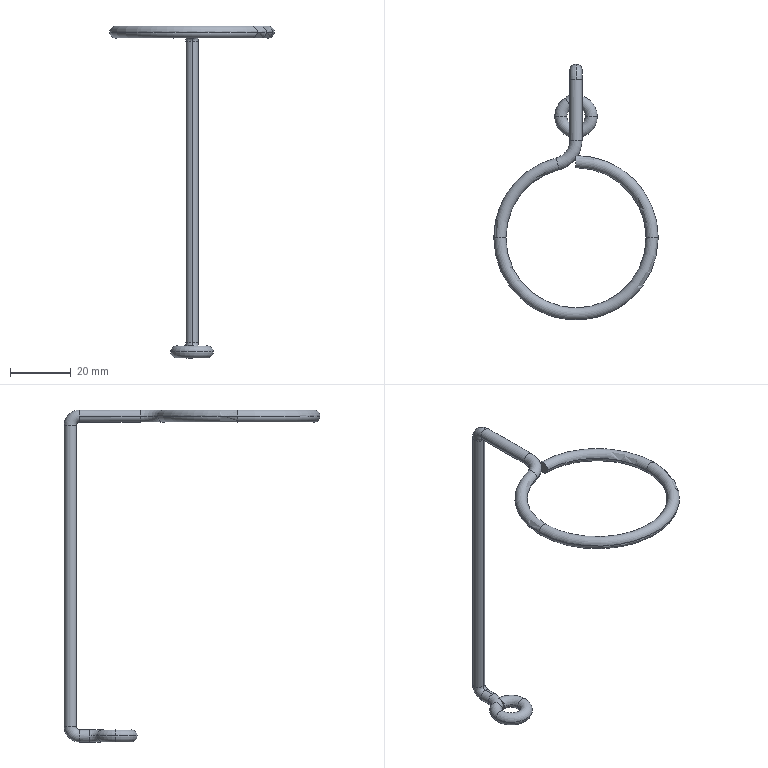Part | SolidWorks | features 3DProfileFeature 2, Sweep 1 | 1 solid | 28 faces | box 54 x 84 x 109 mm | volume 4114 mm3 | torus 20 | cylinder 6 | plane 2 | commonest cylinder face diameters 4 x6
STEP:
#1=CARTESIAN_POINT('',(7.,0.,0.));
#2=VERTEX_POINT('',#1);
#3=CARTESIAN_POINT('',(3.,0.,0.));
#4=VERTEX_POINT('',#3);
#5=CARTESIAN_POINT('',(5.,0.,0.));
#6=DIRECTION('',(0.,-1.,0.));
#7=DIRECTION('',(0.,0.,-1.));
#8=AXIS2_PLACEMENT_3D('',#5,#6,#7);
#9=CIRCLE('',#8,2.);
#10=EDGE_CURVE('',#2,#4,#9,.T.);
#11=ORIENTED_EDGE('',*,*,#10,.F.);
#12=CARTESIAN_POINT('',(0.,7.,0.));
#13=VERTEX_POINT('',#12);
#14=CARTESIAN_POINT('',(0.,0.,0.));
#15=DIRECTION('',(0.,0.,1.));
#16=DIRECTION('',(1.,0.,0.));
#17=AXIS2_PLACEMENT_3D('',#14,#15,#16);
#18=CIRCLE('',#17,7.);
#19=EDGE_CURVE('',#2,#13,#18,.T.);
#20=ORIENTED_EDGE('',*,*,#19,.T.);
#21=CARTESIAN_POINT('',(0.,3.,0.));
#22=VERTEX_POINT('',#21);
#23=CARTESIAN_POINT('',(0.,5.,0.));
#24=DIRECTION('',(1.,0.,0.));
#25=DIRECTION('',(0.,0.,-1.));
#26=AXIS2_PLACEMENT_3D('',#23,#24,#25);
#27=CIRCLE('',#26,2.);
#28=EDGE_CURVE('',#13,#22,#27,.T.);
#29=ORIENTED_EDGE('',*,*,#28,.T.);
#30=CARTESIAN_POINT('',(0.,0.,0.));
#31=DIRECTION('',(0.,0.,1.));
#32=DIRECTION('',(1.,0.,0.));
#33=AXIS2_PLACEMENT_3D('',#30,#31,#32);
#34=CIRCLE('',#33,3.);
#35=EDGE_CURVE('',#4,#22,#34,.T.);
#36=ORIENTED_EDGE('',*,*,#35,.F.);
#37=EDGE_LOOP('',(#11,#20,#29,#36));
#38=FACE_OUTER_BOUND('',#37,.T.);
#39=CARTESIAN_POINT('',(0.,0.,0.));
#40=DIRECTION('',(0.,0.,1.));
#41=DIRECTION('',(1.,0.,0.));
#42=AXIS2_PLACEMENT_3D('',#39,#40,#41);
#43=TOROIDAL_SURFACE('',#42,5.,2.);
#44=ADVANCED_FACE('',(#38),#43,.T.);
#45=CARTESIAN_POINT('',(-3.5,6.062,0.));
#46=VERTEX_POINT('',#45);
#47=CARTESIAN_POINT('',(-1.5,2.598,0.));
#48=VERTEX_POINT('',#47);
#49=CARTESIAN_POINT('',(-2.5,4.33,0.));
#50=DIRECTION('',(0.866,0.5,0.));
#51=DIRECTION('',(0.,0.,-1.));
#52=AXIS2_PLACEMENT_3D('',#49,#50,#51);
#53=CIRCLE('',#52,2.);
#54=EDGE_CURVE('',#46,#48,#53,.T.);
#55=ORIENTED_EDGE('',*,*,#54,.T.);
#56=CARTESIAN_POINT('',(2.,8.66,0.));
#57=VERTEX_POINT('',#56);
#58=CARTESIAN_POINT('',(-5.,8.66,0.));
#59=DIRECTION('',(0.,0.,1.));
#60=DIRECTION('',(1.,0.,0.));
#61=AXIS2_PLACEMENT_3D('',#58,#59,#60);
#62=CIRCLE('',#61,7.);
#63=EDGE_CURVE('',#48,#57,#62,.T.);
#64=ORIENTED_EDGE('',*,*,#63,.T.);
#65=CARTESIAN_POINT('',(0.,8.66,2.));
#66=VERTEX_POINT('',#65);
#67=CARTESIAN_POINT('',(0.,8.66,0.));
#68=DIRECTION('',(0.,1.,0.));
#69=DIRECTION('',(0.,0.,-1.));
#70=AXIS2_PLACEMENT_3D('',#67,#68,#69);
#71=CIRCLE('',#70,2.);
#72=EDGE_CURVE('',#66,#57,#71,.T.);
#73=ORIENTED_EDGE('',*,*,#72,.F.);
#74=CARTESIAN_POINT('',(-2.,8.66,0.));
#75=VERTEX_POINT('',#74);
#76=CARTESIAN_POINT('',(0.,8.66,0.));
#77=DIRECTION('',(0.,1.,0.));
#78=DIRECTION('',(0.,0.,-1.));
#79=AXIS2_PLACEMENT_3D('',#76,#77,#78);
#80=CIRCLE('',#79,2.);
#81=EDGE_CURVE('',#75,#66,#80,.T.);
#82=ORIENTED_EDGE('',*,*,#81,.F.);
#83=CARTESIAN_POINT('',(-5.,8.66,0.));
#84=DIRECTION('',(0.,0.,1.));
#85=DIRECTION('',(1.,0.,0.));
#86=AXIS2_PLACEMENT_3D('',#83,#84,#85);
#87=CIRCLE('',#86,3.);
#88=EDGE_CURVE('',#46,#75,#87,.T.);
#89=ORIENTED_EDGE('',*,*,#88,.F.);
#90=EDGE_LOOP('',(#55,#64,#73,#82,#89));
#91=FACE_OUTER_BOUND('',#90,.T.);
#92=CARTESIAN_POINT('',(-5.,8.66,0.));
#93=DIRECTION('',(0.,0.,1.));
#94=DIRECTION('',(1.,0.,0.));
#95=AXIS2_PLACEMENT_3D('',#92,#93,#94);
#96=TOROIDAL_SURFACE('',#95,5.,2.);
#97=ADVANCED_FACE('',(#91),#96,.T.);
#98=CARTESIAN_POINT('',(0.,12.,2.));
#99=VERTEX_POINT('',#98);
#100=CARTESIAN_POINT('',(0.,12.,-2.));
#101=VERTEX_POINT('',#100);
#102=CARTESIAN_POINT('',(0.,12.,0.));
#103=DIRECTION('',(0.,1.,0.));
#104=DIRECTION('',(0.,0.,-1.));
#105=AXIS2_PLACEMENT_3D('',#102,#103,#104);
#106=CIRCLE('',#105,2.);
#107=EDGE_CURVE('',#99,#101,#106,.T.);
#108=ORIENTED_EDGE('',*,*,#107,.T.);
#109=CARTESIAN_POINT('',(0.,17.,3.));
#110=VERTEX_POINT('',#109);
#111=CARTESIAN_POINT('',(0.,12.,3.));
#112=DIRECTION('',(1.,0.,0.));
#113=DIRECTION('',(0.,0.,-1.));
#114=AXIS2_PLACEMENT_3D('',#111,#112,#113);
#115=CIRCLE('',#114,5.);
#116=EDGE_CURVE('',#101,#110,#115,.T.);
#117=ORIENTED_EDGE('',*,*,#116,.T.);
#118=CARTESIAN_POINT('',(0.,13.,3.));
#119=VERTEX_POINT('',#118);
#120=CARTESIAN_POINT('',(0.,15.,3.));
#121=DIRECTION('',(0.,0.,1.));
#122=DIRECTION('',(0.,1.,0.));
#123=AXIS2_PLACEMENT_3D('',#120,#121,#122);
#124=CIRCLE('',#123,2.);
#125=EDGE_CURVE('',#119,#110,#124,.T.);
#126=ORIENTED_EDGE('',*,*,#125,.F.);
#127=CARTESIAN_POINT('',(0.,12.,3.));
#128=DIRECTION('',(1.,0.,0.));
#129=DIRECTION('',(0.,0.,-1.));
#130=AXIS2_PLACEMENT_3D('',#127,#128,#129);
#131=CIRCLE('',#130,1.);
#132=EDGE_CURVE('',#99,#119,#131,.T.);
#133=ORIENTED_EDGE('',*,*,#132,.F.);
#134=EDGE_LOOP('',(#108,#117,#126,#133));
#135=FACE_OUTER_BOUND('',#134,.T.);
#136=CARTESIAN_POINT('',(0.,12.,3.));
#137=DIRECTION('',(1.,0.,0.));
#138=DIRECTION('',(0.,0.,-1.));
#139=AXIS2_PLACEMENT_3D('',#136,#137,#138);
#140=TOROIDAL_SURFACE('',#139,3.,2.);
#141=ADVANCED_FACE('',(#135),#140,.T.);
#142=CARTESIAN_POINT('',(0.,13.,102.));
#143=VERTEX_POINT('',#142);
#144=CARTESIAN_POINT('',(0.,17.,102.));
#145=VERTEX_POINT('',#144);
#146=CARTESIAN_POINT('',(0.,15.,102.));
#147=DIRECTION('',(0.,0.,1.));
#148=DIRECTION('',(0.,1.,0.));
#149=AXIS2_PLACEMENT_3D('',#146,#147,#148);
#150=CIRCLE('',#149,2.);
#151=EDGE_CURVE('',#143,#145,#150,.T.);
#152=ORIENTED_EDGE('',*,*,#151,.T.);
#153=CARTESIAN_POINT('',(0.,12.,107.));
#154=VERTEX_POINT('',#153);
#155=CARTESIAN_POINT('',(0.,12.,102.));
#156=DIRECTION('',(1.,0.,0.));
#157=DIRECTION('',(0.,0.,-1.));
#158=AXIS2_PLACEMENT_3D('',#155,#156,#157);
#159=CIRCLE('',#158,5.);
#160=EDGE_CURVE('',#145,#154,#159,.T.);
#161=ORIENTED_EDGE('',*,*,#160,.T.);
#162=CARTESIAN_POINT('',(2.,12.,105.));
#163=VERTEX_POINT('',#162);
#164=CARTESIAN_POINT('',(0.,12.,105.));
#165=DIRECTION('',(0.,-1.,0.));
#166=DIRECTION('',(0.,0.,1.));
#167=AXIS2_PLACEMENT_3D('',#164,#165,#166);
#168=CIRCLE('',#167,2.);
#169=EDGE_CURVE('',#163,#154,#168,.T.);
#170=ORIENTED_EDGE('',*,*,#169,.F.);
#171=CARTESIAN_POINT('',(0.,12.,103.));
#172=VERTEX_POINT('',#171);
#173=CARTESIAN_POINT('',(0.,12.,105.));
#174=DIRECTION('',(0.,-1.,0.));
#175=DIRECTION('',(0.,0.,1.));
#176=AXIS2_PLACEMENT_3D('',#173,#174,#175);
#177=CIRCLE('',#176,2.);
#178=EDGE_CURVE('',#172,#163,#177,.T.);
#179=ORIENTED_EDGE('',*,*,#178,.F.);
#180=CARTESIAN_POINT('',(0.,12.,102.));
#181=DIRECTION('',(1.,0.,0.));
#182=DIRECTION('',(0.,0.,-1.));
#183=AXIS2_PLACEMENT_3D('',#180,#181,#182);
#184=CIRCLE('',#183,1.);
#185=EDGE_CURVE('',#143,#172,#184,.T.);
#186=ORIENTED_EDGE('',*,*,#185,.F.);
#187=EDGE_LOOP('',(#152,#161,#170,#179,#186));
#188=FACE_OUTER_BOUND('',#187,.T.);
#189=CARTESIAN_POINT('',(0.,12.,102.));
#190=DIRECTION('',(1.,0.,0.));
#191=DIRECTION('',(0.,0.,-1.));
#192=AXIS2_PLACEMENT_3D('',#189,#190,#191);
#193=TOROIDAL_SURFACE('',#192,3.,2.);
#194=ADVANCED_FACE('',(#188),#193,.T.);
#195=CARTESIAN_POINT('',(-2.,-7.984,105.));
#196=VERTEX_POINT('',#195);
#197=CARTESIAN_POINT('',(2.,-7.984,105.));
#198=VERTEX_POINT('',#197);
#199=CARTESIAN_POINT('',(0.,-7.984,105.));
#200=DIRECTION('',(0.,-1.,0.));
#201=DIRECTION('',(0.,0.,1.));
#202=AXIS2_PLACEMENT_3D('',#199,#200,#201);
#203=CIRCLE('',#202,2.);
#204=EDGE_CURVE('',#196,#198,#203,.T.);
#205=ORIENTED_EDGE('',*,*,#204,.T.);
#206=CARTESIAN_POINT('',(-5.576,-17.686,105.));
#207=VERTEX_POINT('',#206);
#208=CARTESIAN_POINT('',(-8.,-7.984,105.));
#209=DIRECTION('',(0.,0.,-1.));
#210=DIRECTION('',(-1.,0.,0.));
#211=AXIS2_PLACEMENT_3D('',#208,#209,#210);
#212=CIRCLE('',#211,10.);
#213=EDGE_CURVE('',#198,#207,#212,.T.);
#214=ORIENTED_EDGE('',*,*,#213,.T.);
#215=CARTESIAN_POINT('',(-6.545,-13.805,105.));
#216=VERTEX_POINT('',#215);
#217=CARTESIAN_POINT('',(-6.061,-15.746,105.));
#218=DIRECTION('',(-0.9702,-0.2424,0.));
#219=DIRECTION('',(0.,0.,1.));
#220=AXIS2_PLACEMENT_3D('',#217,#218,#219);
#221=CIRCLE('',#220,2.);
#222=EDGE_CURVE('',#216,#207,#221,.T.);
#223=ORIENTED_EDGE('',*,*,#222,.F.);
#224=CARTESIAN_POINT('',(-8.,-7.984,105.));
#225=DIRECTION('',(0.,0.,-1.));
#226=DIRECTION('',(-1.,0.,0.));
#227=AXIS2_PLACEMENT_3D('',#224,#225,#226);
#228=CIRCLE('',#227,6.);
#229=EDGE_CURVE('',#196,#216,#228,.T.);
#230=ORIENTED_EDGE('',*,*,#229,.F.);
#231=EDGE_LOOP('',(#205,#214,#223,#230));
#232=FACE_OUTER_BOUND('',#231,.T.);
#233=CARTESIAN_POINT('',(-8.,-7.984,105.));
#234=DIRECTION('',(0.,0.,-1.));
#235=DIRECTION('',(-1.,0.,0.));
#236=AXIS2_PLACEMENT_3D('',#233,#234,#235);
#237=TOROIDAL_SURFACE('',#236,8.,2.);
#238=ADVANCED_FACE('',(#232),#237,.T.);
#239=CARTESIAN_POINT('',(27.,-40.,105.));
#240=VERTEX_POINT('',#239);
#241=CARTESIAN_POINT('',(23.,-40.,105.));
#242=VERTEX_POINT('',#241);
#243=CARTESIAN_POINT('',(25.,-40.,105.));
#244=DIRECTION('',(0.,-1.,0.));
#245=DIRECTION('',(0.,0.,-1.));
#246=AXIS2_PLACEMENT_3D('',#243,#244,#245);
#247=CIRCLE('',#246,2.);
#248=EDGE_CURVE('',#240,#242,#247,.T.);
#249=ORIENTED_EDGE('',*,*,#248,.F.);
#250=CARTESIAN_POINT('',(0.,-13.,105.));
#251=VERTEX_POINT('',#250);
#252=CARTESIAN_POINT('',(0.,-40.,105.));
#253=DIRECTION('',(0.,0.,1.));
#254=DIRECTION('',(1.,0.,0.));
#255=AXIS2_PLACEMENT_3D('',#252,#253,#254);
#256=CIRCLE('',#255,27.);
#257=EDGE_CURVE('',#240,#251,#256,.T.);
#258=ORIENTED_EDGE('',*,*,#257,.T.);
#259=CARTESIAN_POINT('',(0.,-17.,105.));
#260=VERTEX_POINT('',#259);
#261=CARTESIAN_POINT('',(0.,-15.,105.));
#262=DIRECTION('',(-1.,0.,0.));
#263=DIRECTION('',(0.,0.,1.));
#264=AXIS2_PLACEMENT_3D('',#261,#262,#263);
#265=CIRCLE('',#264,2.);
#266=EDGE_CURVE('',#260,#251,#265,.T.);
#267=ORIENTED_EDGE('',*,*,#266,.F.);
#268=CARTESIAN_POINT('',(0.,-40.,105.));
#269=DIRECTION('',(0.,0.,1.));
#270=DIRECTION('',(1.,0.,0.));
#271=AXIS2_PLACEMENT_3D('',#268,#269,#270);
#272=CIRCLE('',#271,23.);
#273=EDGE_CURVE('',#242,#260,#272,.T.);
#274=ORIENTED_EDGE('',*,*,#273,.F.);
#275=EDGE_LOOP('',(#249,#258,#267,#274));
#276=FACE_OUTER_BOUND('',#275,.T.);
#277=CARTESIAN_POINT('',(0.,-40.,105.));
#278=DIRECTION('',(0.,0.,1.));
#279=DIRECTION('',(1.,0.,0.));
#280=AXIS2_PLACEMENT_3D('',#277,#278,#279);
#281=TOROIDAL_SURFACE('',#280,25.,2.);
#282=ADVANCED_FACE('',(#276),#281,.T.);
#283=CARTESIAN_POINT('',(-27.,-40.,105.));
#284=VERTEX_POINT('',#283);
#285=CARTESIAN_POINT('',(-23.,-40.,105.));
#286=VERTEX_POINT('',#285);
#287=CARTESIAN_POINT('',(-25.,-40.,105.));
#288=DIRECTION('',(0.,1.,0.));
#289=DIRECTION('',(-1.,0.,0.));
#290=AXIS2_PLACEMENT_3D('',#287,#288,#289);
#291=CIRCLE('',#290,2.);
#292=EDGE_CURVE('',#284,#286,#291,.T.);
#293=ORIENTED_EDGE('',*,*,#292,.F.);
#294=CARTESIAN_POINT('',(0.,-40.,105.));
#295=DIRECTION('',(0.,0.,1.));
#296=DIRECTION('',(1.,0.,0.));
#297=AXIS2_PLACEMENT_3D('',#294,#295,#296);
#298=CIRCLE('',#297,27.);
#299=EDGE_CURVE('',#284,#240,#298,.T.);
#300=ORIENTED_EDGE('',*,*,#299,.T.);
#301=ORIENTED_EDGE('',*,*,#248,.T.);
#302=CARTESIAN_POINT('',(0.,-40.,105.));
#303=DIRECTION('',(0.,0.,1.));
#304=DIRECTION('',(1.,0.,0.));
#305=AXIS2_PLACEMENT_3D('',#302,#303,#304);
#306=CIRCLE('',#305,23.);
#307=EDGE_CURVE('',#286,#242,#306,.T.);
#308=ORIENTED_EDGE('',*,*,#307,.F.);
#309=EDGE_LOOP('',(#293,#300,#301,#308));
#310=FACE_OUTER_BOUND('',#309,.T.);
#311=CARTESIAN_POINT('',(0.,-40.,105.));
#312=DIRECTION('',(0.,0.,1.));
#313=DIRECTION('',(1.,0.,0.));
#314=AXIS2_PLACEMENT_3D('',#311,#312,#313);
#315=TOROIDAL_SURFACE('',#314,25.,2.);
#316=ADVANCED_FACE('',(#310),#315,.T.);
#317=CARTESIAN_POINT('',(-6.061,-15.746,105.));
#318=DIRECTION('',(-0.9702,-0.2424,0.));
#319=DIRECTION('',(0.,0.,1.));
#320=AXIS2_PLACEMENT_3D('',#317,#318,#319);
#321=CIRCLE('',#320,2.);
#322=EDGE_CURVE('',#207,#216,#321,.T.);
#323=ORIENTED_EDGE('',*,*,#322,.T.);
#324=CARTESIAN_POINT('',(0.,-40.,105.));
#325=DIRECTION('',(0.,0.,1.));
#326=DIRECTION('',(1.,0.,0.));
#327=AXIS2_PLACEMENT_3D('',#324,#325,#326);
#328=CIRCLE('',#327,27.);
#329=EDGE_CURVE('',#216,#284,#328,.T.);
#330=ORIENTED_EDGE('',*,*,#329,.T.);
#331=ORIENTED_EDGE('',*,*,#292,.T.);
#332=CARTESIAN_POINT('',(0.,-40.,105.));
#333=DIRECTION('',(0.,0.,1.));
#334=DIRECTION('',(1.,0.,0.));
#335=AXIS2_PLACEMENT_3D('',#332,#333,#334);
#336=CIRCLE('',#335,23.);
#337=EDGE_CURVE('',#207,#286,#336,.T.);
#338=ORIENTED_EDGE('',*,*,#337,.F.);
#339=EDGE_LOOP('',(#323,#330,#331,#338));
#340=FACE_OUTER_BOUND('',#339,.T.);
#341=CARTESIAN_POINT('',(0.,-40.,105.));
#342=DIRECTION('',(0.,0.,1.));
#343=DIRECTION('',(1.,0.,0.));
#344=AXIS2_PLACEMENT_3D('',#341,#342,#343);
#345=TOROIDAL_SURFACE('',#344,25.,2.);
#346=ADVANCED_FACE('',(#340),#345,.T.);
#347=CARTESIAN_POINT('',(-7.,0.,0.));
#348=VERTEX_POINT('',#347);
#349=CARTESIAN_POINT('',(-3.,0.,0.));
#350=VERTEX_POINT('',#349);
#351=CARTESIAN_POINT('',(-5.,0.,0.));
#352=DIRECTION('',(0.,1.,0.));
#353=DIRECTION('',(-1.,0.,0.));
#354=AXIS2_PLACEMENT_3D('',#351,#352,#353);
#355=CIRCLE('',#354,2.);
#356=EDGE_CURVE('',#348,#350,#355,.T.);
#357=ORIENTED_EDGE('',*,*,#356,.F.);
#358=CARTESIAN_POINT('',(0.,0.,0.));
#359=DIRECTION('',(0.,0.,1.));
#360=DIRECTION('',(1.,0.,0.));
#361=AXIS2_PLACEMENT_3D('',#358,#359,#360);
#362=CIRCLE('',#361,7.);
#363=EDGE_CURVE('',#348,#2,#362,.T.);
#364=ORIENTED_EDGE('',*,*,#363,.T.);
#365=ORIENTED_EDGE('',*,*,#10,.T.);
#366=CARTESIAN_POINT('',(0.,0.,0.));
#367=DIRECTION('',(0.,0.,1.));
#368=DIRECTION('',(1.,0.,0.));
#369=AXIS2_PLACEMENT_3D('',#366,#367,#368);
#370=CIRCLE('',#369,3.);
#371=EDGE_CURVE('',#350,#4,#370,.T.);
#372=ORIENTED_EDGE('',*,*,#371,.F.);
#373=EDGE_LOOP('',(#357,#364,#365,#372));
#374=FACE_OUTER_BOUND('',#373,.T.);
#375=CARTESIAN_POINT('',(0.,0.,0.));
#376=DIRECTION('',(0.,0.,1.));
#377=DIRECTION('',(1.,0.,0.));
#378=AXIS2_PLACEMENT_3D('',#375,#376,#377);
#379=TOROIDAL_SURFACE('',#378,5.,2.);
#380=ADVANCED_FACE('',(#374),#379,.T.);
#381=ORIENTED_EDGE('',*,*,#54,.F.);
#382=CARTESIAN_POINT('',(0.,0.,0.));
#383=DIRECTION('',(0.,0.,1.));
#384=DIRECTION('',(1.,0.,0.));
#385=AXIS2_PLACEMENT_3D('',#382,#383,#384);
#386=CIRCLE('',#385,7.);
#387=EDGE_CURVE('',#46,#348,#386,.T.);
#388=ORIENTED_EDGE('',*,*,#387,.T.);
#389=ORIENTED_EDGE('',*,*,#356,.T.);
#390=CARTESIAN_POINT('',(0.,0.,0.));
#391=DIRECTION('',(0.,0.,1.));
#392=DIRECTION('',(1.,0.,0.));
#393=AXIS2_PLACEMENT_3D('',#390,#391,#392);
#394=CIRCLE('',#393,3.);
#395=EDGE_CURVE('',#48,#350,#394,.T.);
#396=ORIENTED_EDGE('',*,*,#395,.F.);
#397=EDGE_LOOP('',(#381,#388,#389,#396));
#398=FACE_OUTER_BOUND('',#397,.T.);
#399=CARTESIAN_POINT('',(0.,0.,0.));
#400=DIRECTION('',(0.,0.,1.));
#401=DIRECTION('',(1.,0.,0.));
#402=AXIS2_PLACEMENT_3D('',#399,#400,#401);
#403=TOROIDAL_SURFACE('',#402,5.,2.);
#404=ADVANCED_FACE('',(#398),#403,.T.);
#405=ORIENTED_EDGE('',*,*,#387,.F.);
#406=CARTESIAN_POINT('',(-2.5,4.33,0.));
#407=DIRECTION('',(0.866,0.5,0.));
#408=DIRECTION('',(0.,0.,-1.));
#409=AXIS2_PLACEMENT_3D('',#406,#407,#408);
#410=CIRCLE('',#409,2.);
#411=EDGE_CURVE('',#48,#46,#410,.T.);
#412=ORIENTED_EDGE('',*,*,#411,.F.);
#413=ORIENTED_EDGE('',*,*,#395,.T.);
#414=CARTESIAN_POINT('',(-5.,0.,0.));
#415=DIRECTION('',(0.,1.,0.));
#416=DIRECTION('',(-1.,0.,0.));
#417=AXIS2_PLACEMENT_3D('',#414,#415,#416);
#418=CIRCLE('',#417,2.);
#419=EDGE_CURVE('',#350,#348,#418,.T.);
#420=ORIENTED_EDGE('',*,*,#419,.T.);
#421=EDGE_LOOP('',(#405,#412,#413,#420));
#422=FACE_OUTER_BOUND('',#421,.T.);
#423=CARTESIAN_POINT('',(0.,0.,0.));
#424=DIRECTION('',(0.,0.,1.));
#425=DIRECTION('',(1.,0.,0.));
#426=AXIS2_PLACEMENT_3D('',#423,#424,#425);
#427=TOROIDAL_SURFACE('',#426,5.,2.);
#428=ADVANCED_FACE('',(#422),#427,.T.);
#429=ORIENTED_EDGE('',*,*,#363,.F.);
#430=ORIENTED_EDGE('',*,*,#419,.F.);
#431=ORIENTED_EDGE('',*,*,#371,.T.);
#432=CARTESIAN_POINT('',(5.,0.,0.));
#433=DIRECTION('',(0.,-1.,0.));
#434=DIRECTION('',(0.,0.,-1.));
#435=AXIS2_PLACEMENT_3D('',#432,#433,#434);
#436=CIRCLE('',#435,2.);
#437=EDGE_CURVE('',#4,#2,#436,.T.);
#438=ORIENTED_EDGE('',*,*,#437,.T.);
#439=EDGE_LOOP('',(#429,#430,#431,#438));
#440=FACE_OUTER_BOUND('',#439,.T.);
#441=CARTESIAN_POINT('',(0.,0.,0.));
#442=DIRECTION('',(0.,0.,1.));
#443=DIRECTION('',(1.,0.,0.));
#444=AXIS2_PLACEMENT_3D('',#441,#442,#443);
#445=TOROIDAL_SURFACE('',#444,5.,2.);
#446=ADVANCED_FACE('',(#440),#445,.T.);
#447=ORIENTED_EDGE('',*,*,#72,.T.);
#448=CARTESIAN_POINT('',(0.,8.66,-2.));
#449=VERTEX_POINT('',#448);
#450=CARTESIAN_POINT('',(0.,8.66,0.));
#451=DIRECTION('',(0.,1.,0.));
#452=DIRECTION('',(0.,0.,-1.));
#453=AXIS2_PLACEMENT_3D('',#450,#451,#452);
#454=CIRCLE('',#453,2.);
#455=EDGE_CURVE('',#57,#449,#454,.T.);
#456=ORIENTED_EDGE('',*,*,#455,.T.);
#457=CARTESIAN_POINT('',(0.,8.66,-2.));
#458=DIRECTION('',(0.,1.,0.));
#459=VECTOR('',#458,1000.);
#460=LINE('',#457,#459);
#461=EDGE_CURVE('',#449,#101,#460,.T.);
#462=ORIENTED_EDGE('',*,*,#461,.T.);
#463=ORIENTED_EDGE('',*,*,#107,.F.);
#464=CARTESIAN_POINT('',(0.,8.66,2.));
#465=DIRECTION('',(0.,1.,0.));
#466=VECTOR('',#465,1000.);
#467=LINE('',#464,#466);
#468=EDGE_CURVE('',#66,#99,#467,.T.);
#469=ORIENTED_EDGE('',*,*,#468,.F.);
#470=EDGE_LOOP('',(#447,#456,#462,#463,#469));
#471=FACE_OUTER_BOUND('',#470,.T.);
#472=CARTESIAN_POINT('',(0.,8.66,0.));
#473=DIRECTION('',(0.,1.,0.));
#474=DIRECTION('',(0.,0.,1.));
#475=AXIS2_PLACEMENT_3D('',#472,#473,#474);
#476=CYLINDRICAL_SURFACE('',#475,2.);
#477=ADVANCED_FACE('',(#471),#476,.T.);
#478=ORIENTED_EDGE('',*,*,#125,.T.);
#479=CARTESIAN_POINT('',(0.,17.,3.));
#480=DIRECTION('',(0.,0.,1.));
#481=VECTOR('',#480,1000.);
#482=LINE('',#479,#481);
#483=EDGE_CURVE('',#110,#145,#482,.T.);
#484=ORIENTED_EDGE('',*,*,#483,.T.);
#485=ORIENTED_EDGE('',*,*,#151,.F.);
#486=CARTESIAN_POINT('',(0.,13.,3.));
#487=DIRECTION('',(0.,0.,1.));
#488=VECTOR('',#487,1000.);
#489=LINE('',#486,#488);
#490=EDGE_CURVE('',#119,#143,#489,.T.);
#491=ORIENTED_EDGE('',*,*,#490,.F.);
#492=EDGE_LOOP('',(#478,#484,#485,#491));
#493=FACE_OUTER_BOUND('',#492,.T.);
#494=CARTESIAN_POINT('',(0.,15.,3.));
#495=DIRECTION('',(0.,0.,1.));
#496=DIRECTION('',(0.,-1.,0.));
#497=AXIS2_PLACEMENT_3D('',#494,#495,#496);
#498=CYLINDRICAL_SURFACE('',#497,2.);
#499=ADVANCED_FACE('',(#493),#498,.T.);
#500=ORIENTED_EDGE('',*,*,#169,.T.);
#501=CARTESIAN_POINT('',(-2.,12.,105.));
#502=VERTEX_POINT('',#501);
#503=CARTESIAN_POINT('',(0.,12.,105.));
#504=DIRECTION('',(0.,-1.,0.));
#505=DIRECTION('',(0.,0.,1.));
#506=AXIS2_PLACEMENT_3D('',#503,#504,#505);
#507=CIRCLE('',#506,2.);
#508=EDGE_CURVE('',#154,#502,#507,.T.);
#509=ORIENTED_EDGE('',*,*,#508,.T.);
#510=CARTESIAN_POINT('',(-2.,12.,105.));
#511=DIRECTION('',(0.,-1.,0.));
#512=VECTOR('',#511,1000.);
#513=LINE('',#510,#512);
#514=EDGE_CURVE('',#502,#196,#513,.T.);
#515=ORIENTED_EDGE('',*,*,#514,.T.);
#516=CARTESIAN_POINT('',(0.,-7.984,105.));
#517=DIRECTION('',(0.,-1.,0.));
#518=DIRECTION('',(0.,0.,1.));
#519=AXIS2_PLACEMENT_3D('',#516,#517,#518);
#520=CIRCLE('',#519,2.);
#521=EDGE_CURVE('',#198,#196,#520,.T.);
#522=ORIENTED_EDGE('',*,*,#521,.F.);
#523=CARTESIAN_POINT('',(2.,12.,105.));
#524=DIRECTION('',(0.,-1.,0.));
#525=VECTOR('',#524,1000.);
#526=LINE('',#523,#525);
#527=EDGE_CURVE('',#163,#198,#526,.T.);
#528=ORIENTED_EDGE('',*,*,#527,.F.);
#529=EDGE_LOOP('',(#500,#509,#515,#522,#528));
#530=FACE_OUTER_BOUND('',#529,.T.);
#531=CARTESIAN_POINT('',(0.,12.,105.));
#532=DIRECTION('',(0.,-1.,0.));
#533=DIRECTION('',(1.,0.,0.));
#534=AXIS2_PLACEMENT_3D('',#531,#532,#533);
#535=CYLINDRICAL_SURFACE('',#534,2.);
#536=ADVANCED_FACE('',(#530),#535,.T.);
#537=ORIENTED_EDGE('',*,*,#329,.F.);
#538=ORIENTED_EDGE('',*,*,#222,.T.);
#539=ORIENTED_EDGE('',*,*,#337,.T.);
#540=CARTESIAN_POINT('',(-25.,-40.,105.));
#541=DIRECTION('',(0.,1.,0.));
#542=DIRECTION('',(-1.,0.,0.));
#543=AXIS2_PLACEMENT_3D('',#540,#541,#542);
#544=CIRCLE('',#543,2.);
#545=EDGE_CURVE('',#286,#284,#544,.T.);
#546=ORIENTED_EDGE('',*,*,#545,.T.);
#547=EDGE_LOOP('',(#537,#538,#539,#546));
#548=FACE_OUTER_BOUND('',#547,.T.);
#549=CARTESIAN_POINT('',(0.,-40.,105.));
#550=DIRECTION('',(0.,0.,1.));
#551=DIRECTION('',(1.,0.,0.));
#552=AXIS2_PLACEMENT_3D('',#549,#550,#551);
#553=TOROIDAL_SURFACE('',#552,25.,2.);
#554=ADVANCED_FACE('',(#548),#553,.T.);
#555=ORIENTED_EDGE('',*,*,#299,.F.);
#556=ORIENTED_EDGE('',*,*,#545,.F.);
#557=ORIENTED_EDGE('',*,*,#307,.T.);
#558=CARTESIAN_POINT('',(25.,-40.,105.));
#559=DIRECTION('',(0.,-1.,0.));
#560=DIRECTION('',(0.,0.,-1.));
#561=AXIS2_PLACEMENT_3D('',#558,#559,#560);
#562=CIRCLE('',#561,2.);
#563=EDGE_CURVE('',#242,#240,#562,.T.);
#564=ORIENTED_EDGE('',*,*,#563,.T.);
#565=EDGE_LOOP('',(#555,#556,#557,#564));
#566=FACE_OUTER_BOUND('',#565,.T.);
#567=CARTESIAN_POINT('',(0.,-40.,105.));
#568=DIRECTION('',(0.,0.,1.));
#569=DIRECTION('',(1.,0.,0.));
#570=AXIS2_PLACEMENT_3D('',#567,#568,#569);
#571=TOROIDAL_SURFACE('',#570,25.,2.);
#572=ADVANCED_FACE('',(#566),#571,.T.);
#573=ORIENTED_EDGE('',*,*,#257,.F.);
#574=ORIENTED_EDGE('',*,*,#563,.F.);
#575=ORIENTED_EDGE('',*,*,#273,.T.);
#576=CARTESIAN_POINT('',(0.,-15.,105.));
#577=DIRECTION('',(-1.,0.,0.));
#578=DIRECTION('',(0.,0.,1.));
#579=AXIS2_PLACEMENT_3D('',#576,#577,#578);
#580=CIRCLE('',#579,2.);
#581=EDGE_CURVE('',#251,#260,#580,.T.);
#582=ORIENTED_EDGE('',*,*,#581,.F.);
#583=EDGE_LOOP('',(#573,#574,#575,#582));
#584=FACE_OUTER_BOUND('',#583,.T.);
#585=CARTESIAN_POINT('',(0.,-40.,105.));
#586=DIRECTION('',(0.,0.,1.));
#587=DIRECTION('',(1.,0.,0.));
#588=AXIS2_PLACEMENT_3D('',#585,#586,#587);
#589=TOROIDAL_SURFACE('',#588,25.,2.);
#590=ADVANCED_FACE('',(#584),#589,.T.);
#591=ORIENTED_EDGE('',*,*,#213,.F.);
#592=ORIENTED_EDGE('',*,*,#521,.T.);
#593=ORIENTED_EDGE('',*,*,#229,.T.);
#594=ORIENTED_EDGE('',*,*,#322,.F.);
#595=EDGE_LOOP('',(#591,#592,#593,#594));
#596=FACE_OUTER_BOUND('',#595,.T.);
#597=CARTESIAN_POINT('',(-8.,-7.984,105.));
#598=DIRECTION('',(0.,0.,-1.));
#599=DIRECTION('',(-1.,0.,0.));
#600=AXIS2_PLACEMENT_3D('',#597,#598,#599);
#601=TOROIDAL_SURFACE('',#600,8.,2.);
#602=ADVANCED_FACE('',(#596),#601,.T.);
#603=ORIENTED_EDGE('',*,*,#514,.F.);
#604=CARTESIAN_POINT('',(0.,12.,105.));
#605=DIRECTION('',(0.,-1.,0.));
#606=DIRECTION('',(0.,0.,1.));
#607=AXIS2_PLACEMENT_3D('',#604,#605,#606);
#608=CIRCLE('',#607,2.);
#609=EDGE_CURVE('',#502,#172,#608,.T.);
#610=ORIENTED_EDGE('',*,*,#609,.T.);
#611=ORIENTED_EDGE('',*,*,#178,.T.);
#612=ORIENTED_EDGE('',*,*,#527,.T.);
#613=ORIENTED_EDGE('',*,*,#204,.F.);
#614=EDGE_LOOP('',(#603,#610,#611,#612,#613));
#615=FACE_OUTER_BOUND('',#614,.T.);
#616=CARTESIAN_POINT('',(0.,12.,105.));
#617=DIRECTION('',(0.,-1.,0.));
#618=DIRECTION('',(1.,0.,0.));
#619=AXIS2_PLACEMENT_3D('',#616,#617,#618);
#620=CYLINDRICAL_SURFACE('',#619,2.);
#621=ADVANCED_FACE('',(#615),#620,.T.);
#622=ORIENTED_EDGE('',*,*,#160,.F.);
#623=CARTESIAN_POINT('',(0.,15.,102.));
#624=DIRECTION('',(0.,0.,1.));
#625=DIRECTION('',(0.,1.,0.));
#626=AXIS2_PLACEMENT_3D('',#623,#624,#625);
#627=CIRCLE('',#626,2.);
#628=EDGE_CURVE('',#145,#143,#627,.T.);
#629=ORIENTED_EDGE('',*,*,#628,.T.);
#630=ORIENTED_EDGE('',*,*,#185,.T.);
#631=ORIENTED_EDGE('',*,*,#609,.F.);
#632=ORIENTED_EDGE('',*,*,#508,.F.);
#633=EDGE_LOOP('',(#622,#629,#630,#631,#632));
#634=FACE_OUTER_BOUND('',#633,.T.);
#635=CARTESIAN_POINT('',(0.,12.,102.));
#636=DIRECTION('',(1.,0.,0.));
#637=DIRECTION('',(0.,0.,-1.));
#638=AXIS2_PLACEMENT_3D('',#635,#636,#637);
#639=TOROIDAL_SURFACE('',#638,3.,2.);
#640=ADVANCED_FACE('',(#634),#639,.T.);
#641=ORIENTED_EDGE('',*,*,#483,.F.);
#642=CARTESIAN_POINT('',(0.,15.,3.));
#643=DIRECTION('',(0.,0.,1.));
#644=DIRECTION('',(0.,1.,0.));
#645=AXIS2_PLACEMENT_3D('',#642,#643,#644);
#646=CIRCLE('',#645,2.);
#647=EDGE_CURVE('',#110,#119,#646,.T.);
#648=ORIENTED_EDGE('',*,*,#647,.T.);
#649=ORIENTED_EDGE('',*,*,#490,.T.);
#650=ORIENTED_EDGE('',*,*,#628,.F.);
#651=EDGE_LOOP('',(#641,#648,#649,#650));
#652=FACE_OUTER_BOUND('',#651,.T.);
#653=CARTESIAN_POINT('',(0.,15.,3.));
#654=DIRECTION('',(0.,0.,1.));
#655=DIRECTION('',(0.,-1.,0.));
#656=AXIS2_PLACEMENT_3D('',#653,#654,#655);
#657=CYLINDRICAL_SURFACE('',#656,2.);
#658=ADVANCED_FACE('',(#652),#657,.T.);
#659=ORIENTED_EDGE('',*,*,#116,.F.);
#660=CARTESIAN_POINT('',(0.,12.,0.));
#661=DIRECTION('',(0.,1.,0.));
#662=DIRECTION('',(0.,0.,-1.));
#663=AXIS2_PLACEMENT_3D('',#660,#661,#662);
#664=CIRCLE('',#663,2.);
#665=EDGE_CURVE('',#101,#99,#664,.T.);
#666=ORIENTED_EDGE('',*,*,#665,.T.);
#667=ORIENTED_EDGE('',*,*,#132,.T.);
#668=ORIENTED_EDGE('',*,*,#647,.F.);
#669=EDGE_LOOP('',(#659,#666,#667,#668));
#670=FACE_OUTER_BOUND('',#669,.T.);
#671=CARTESIAN_POINT('',(0.,12.,3.));
#672=DIRECTION('',(1.,0.,0.));
#673=DIRECTION('',(0.,0.,-1.));
#674=AXIS2_PLACEMENT_3D('',#671,#672,#673);
#675=TOROIDAL_SURFACE('',#674,3.,2.);
#676=ADVANCED_FACE('',(#670),#675,.T.);
#677=ORIENTED_EDGE('',*,*,#461,.F.);
#678=CARTESIAN_POINT('',(0.,8.66,0.));
#679=DIRECTION('',(0.,1.,0.));
#680=DIRECTION('',(0.,0.,-1.));
#681=AXIS2_PLACEMENT_3D('',#678,#679,#680);
#682=CIRCLE('',#681,2.);
#683=EDGE_CURVE('',#449,#75,#682,.T.);
#684=ORIENTED_EDGE('',*,*,#683,.T.);
#685=ORIENTED_EDGE('',*,*,#81,.T.);
#686=ORIENTED_EDGE('',*,*,#468,.T.);
#687=ORIENTED_EDGE('',*,*,#665,.F.);
#688=EDGE_LOOP('',(#677,#684,#685,#686,#687));
#689=FACE_OUTER_BOUND('',#688,.T.);
#690=CARTESIAN_POINT('',(0.,8.66,0.));
#691=DIRECTION('',(0.,1.,0.));
#692=DIRECTION('',(0.,0.,1.));
#693=AXIS2_PLACEMENT_3D('',#690,#691,#692);
#694=CYLINDRICAL_SURFACE('',#693,2.);
#695=ADVANCED_FACE('',(#689),#694,.T.);
#696=ORIENTED_EDGE('',*,*,#63,.F.);
#697=ORIENTED_EDGE('',*,*,#411,.T.);
#698=ORIENTED_EDGE('',*,*,#88,.T.);
#699=ORIENTED_EDGE('',*,*,#683,.F.);
#700=ORIENTED_EDGE('',*,*,#455,.F.);
#701=EDGE_LOOP('',(#696,#697,#698,#699,#700));
#702=FACE_OUTER_BOUND('',#701,.T.);
#703=CARTESIAN_POINT('',(-5.,8.66,0.));
#704=DIRECTION('',(0.,0.,1.));
#705=DIRECTION('',(1.,0.,0.));
#706=AXIS2_PLACEMENT_3D('',#703,#704,#705);
#707=TOROIDAL_SURFACE('',#706,5.,2.);
#708=ADVANCED_FACE('',(#702),#707,.T.);
#709=ORIENTED_EDGE('',*,*,#19,.F.);
#710=ORIENTED_EDGE('',*,*,#437,.F.);
#711=ORIENTED_EDGE('',*,*,#35,.T.);
#712=CARTESIAN_POINT('',(0.,5.,0.));
#713=DIRECTION('',(1.,0.,0.));
#714=DIRECTION('',(0.,0.,-1.));
#715=AXIS2_PLACEMENT_3D('',#712,#713,#714);
#716=CIRCLE('',#715,2.);
#717=EDGE_CURVE('',#22,#13,#716,.T.);
#718=ORIENTED_EDGE('',*,*,#717,.T.);
#719=EDGE_LOOP('',(#709,#710,#711,#718));
#720=FACE_OUTER_BOUND('',#719,.T.);
#721=CARTESIAN_POINT('',(0.,0.,0.));
#722=DIRECTION('',(0.,0.,1.));
#723=DIRECTION('',(1.,0.,0.));
#724=AXIS2_PLACEMENT_3D('',#721,#722,#723);
#725=TOROIDAL_SURFACE('',#724,5.,2.);
#726=ADVANCED_FACE('',(#720),#725,.T.);
#727=ORIENTED_EDGE('',*,*,#266,.T.);
#728=ORIENTED_EDGE('',*,*,#581,.T.);
#729=EDGE_LOOP('',(#727,#728));
#730=FACE_OUTER_BOUND('',#729,.T.);
#731=CARTESIAN_POINT('',(0.,-15.,105.));
#732=DIRECTION('',(-1.,0.,0.));
#733=DIRECTION('',(0.,0.,1.));
#734=AXIS2_PLACEMENT_3D('',#731,#732,#733);
#735=PLANE('',#734);
#736=ADVANCED_FACE('',(#730),#735,.T.);
#737=ORIENTED_EDGE('',*,*,#717,.F.);
#738=ORIENTED_EDGE('',*,*,#28,.F.);
#739=EDGE_LOOP('',(#737,#738));
#740=FACE_OUTER_BOUND('',#739,.T.);
#741=CARTESIAN_POINT('',(0.,5.,0.));
#742=DIRECTION('',(1.,0.,0.));
#743=DIRECTION('',(0.,0.,-1.));
#744=AXIS2_PLACEMENT_3D('',#741,#742,#743);
#745=PLANE('',#744);
#746=ADVANCED_FACE('',(#740),#745,.F.);
#747=CLOSED_SHELL('',(#44,#97,#141,#194,#238,#282,#316,#346,#380,#404,#428,#446,#477,#499,#536,#554,#572,#590,#602,#621,#640,#658,#676,#695,#708,#726,#736,#746));
#748=MANIFOLD_SOLID_BREP('',#747);
#749=CARTESIAN_POINT('',(0.,0.,0.));
#750=DIRECTION('',(0.,0.,1.));
#751=DIRECTION('',(1.,0.,0.));
#752=AXIS2_PLACEMENT_3D('',#749,#750,#751);
#753=(LENGTH_UNIT()NAMED_UNIT(*)SI_UNIT(.MILLI.,.METRE.));
#754=UNCERTAINTY_MEASURE_WITH_UNIT(LENGTH_MEASURE(0.00001),#753,'','');
#755=(NAMED_UNIT(*)PLANE_ANGLE_UNIT()SI_UNIT($,.RADIAN.));
#756=(NAMED_UNIT(*)SI_UNIT($,.STERADIAN.)SOLID_ANGLE_UNIT());
#757=(GEOMETRIC_REPRESENTATION_CONTEXT(3)GLOBAL_UNCERTAINTY_ASSIGNED_CONTEXT((#754))GLOBAL_UNIT_ASSIGNED_CONTEXT((#753,#755,#756))REPRESENTATION_CONTEXT('',''));
#758=ADVANCED_BREP_SHAPE_REPRESENTATION('',(#748,#752),#757);